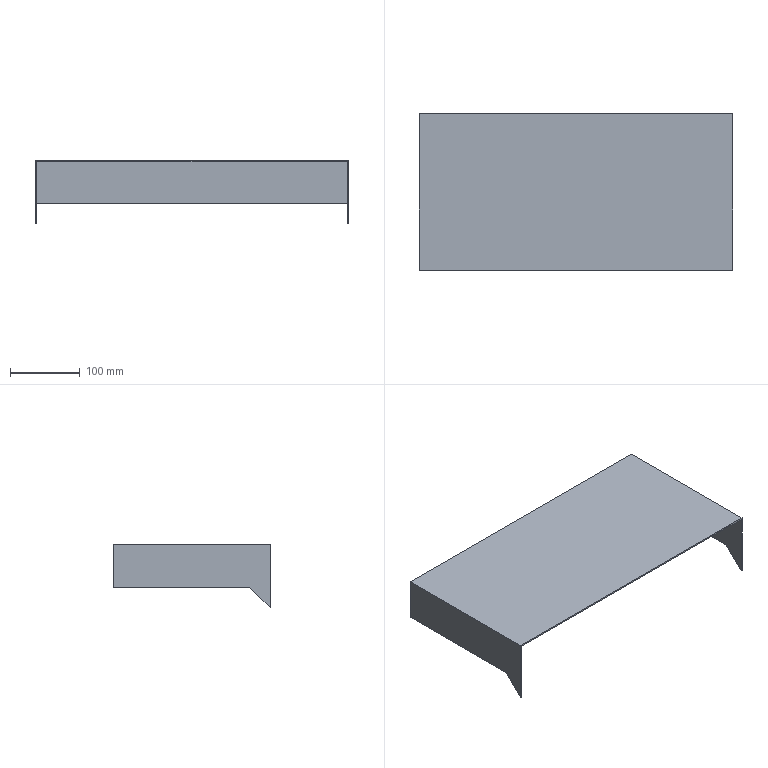Part | Creo | features PROTRUSION 5, CURVE 4, DATUM PLANE 3, COORDINATE SYSTEM 1, MIRROR 1 | 1 solid | 12 faces | box 450 x 225 x 92 mm | volume 311820 mm3 | plane 12
STEP:
#1=CARTESIAN_POINT('',(0.,0.,0.));
#2=DIRECTION('',(0.,0.,1.));
#3=DIRECTION('',(1.,0.,0.));
#4=AXIS2_PLACEMENT_3D('',#1,#2,#3);
#5=CARTESIAN_POINT('',(-223.,95.5,0.));
#6=VERTEX_POINT('',#5);
#7=CARTESIAN_POINT('',(-223.,-127.5,0.));
#8=VERTEX_POINT('',#7);
#9=CARTESIAN_POINT('',(-223.,95.5,0.));
#10=DIRECTION('',(0.,-1.,0.));
#11=VECTOR('',#10,223.);
#12=LINE('',#9,#11);
#13=EDGE_CURVE('',#6,#8,#12,.T.);
#14=ORIENTED_EDGE('',*,*,#13,.T.);
#15=CARTESIAN_POINT('',(223.,-127.5,0.));
#16=VERTEX_POINT('',#15);
#17=CARTESIAN_POINT('',(-223.,-127.5,0.));
#18=DIRECTION('',(1.,0.,0.));
#19=VECTOR('',#18,446.);
#20=LINE('',#17,#19);
#21=EDGE_CURVE('',#8,#16,#20,.T.);
#22=ORIENTED_EDGE('',*,*,#21,.T.);
#23=CARTESIAN_POINT('',(223.,95.5,0.));
#24=VERTEX_POINT('',#23);
#25=CARTESIAN_POINT('',(223.,-127.5,0.));
#26=DIRECTION('',(0.,1.,0.));
#27=VECTOR('',#26,223.);
#28=LINE('',#25,#27);
#29=EDGE_CURVE('',#16,#24,#28,.T.);
#30=ORIENTED_EDGE('',*,*,#29,.T.);
#31=CARTESIAN_POINT('',(223.,95.5,0.));
#32=DIRECTION('',(-1.,0.,0.));
#33=VECTOR('',#32,446.);
#34=LINE('',#31,#33);
#35=EDGE_CURVE('',#24,#6,#34,.T.);
#36=ORIENTED_EDGE('',*,*,#35,.T.);
#37=EDGE_LOOP('',(#14,#22,#30,#36));
#38=FACE_OUTER_BOUND('',#37,.F.);
#39=CARTESIAN_POINT('',(0.,0.,0.));
#40=DIRECTION('',(0.,0.,1.));
#41=DIRECTION('',(1.,0.,0.));
#42=AXIS2_PLACEMENT_3D('',#39,#40,#41);
#43=PLANE('',#42);
#44=ADVANCED_FACE('',(#38),#43,.F.);
#45=ORIENTED_EDGE('',*,*,#13,.F.);
#46=CARTESIAN_POINT('',(-223.,95.5,-60.));
#47=VERTEX_POINT('',#46);
#48=CARTESIAN_POINT('',(-223.,95.5,0.));
#49=DIRECTION('',(0.,0.,-1.));
#50=VECTOR('',#49,60.);
#51=LINE('',#48,#50);
#52=EDGE_CURVE('',#6,#47,#51,.T.);
#53=ORIENTED_EDGE('',*,*,#52,.T.);
#54=CARTESIAN_POINT('',(-223.,-97.5,-60.));
#55=VERTEX_POINT('',#54);
#56=CARTESIAN_POINT('',(-223.,95.5,-60.));
#57=DIRECTION('',(0.,-1.,0.));
#58=VECTOR('',#57,193.);
#59=LINE('',#56,#58);
#60=EDGE_CURVE('',#47,#55,#59,.T.);
#61=ORIENTED_EDGE('',*,*,#60,.T.);
#62=CARTESIAN_POINT('',(-223.,-127.5,-90.));
#63=VERTEX_POINT('',#62);
#64=CARTESIAN_POINT('',(-223.,-97.5,-60.));
#65=DIRECTION('',(0.,-0.7071,-0.7071));
#66=VECTOR('',#65,42.426);
#67=LINE('',#64,#66);
#68=EDGE_CURVE('',#55,#63,#67,.T.);
#69=ORIENTED_EDGE('',*,*,#68,.T.);
#70=CARTESIAN_POINT('',(-223.,-127.5,-90.));
#71=DIRECTION('',(0.,0.,1.));
#72=VECTOR('',#71,90.);
#73=LINE('',#70,#72);
#74=EDGE_CURVE('',#63,#8,#73,.T.);
#75=ORIENTED_EDGE('',*,*,#74,.T.);
#76=EDGE_LOOP('',(#45,#53,#61,#69,#75));
#77=FACE_OUTER_BOUND('',#76,.F.);
#78=CARTESIAN_POINT('',(-223.,95.5,0.));
#79=DIRECTION('',(1.,0.,0.));
#80=DIRECTION('',(0.,-1.,0.));
#81=AXIS2_PLACEMENT_3D('',#78,#79,#80);
#82=PLANE('',#81);
#83=ADVANCED_FACE('',(#77),#82,.T.);
#84=ORIENTED_EDGE('',*,*,#35,.F.);
#85=CARTESIAN_POINT('',(223.,95.5,-60.));
#86=VERTEX_POINT('',#85);
#87=CARTESIAN_POINT('',(223.,95.5,0.));
#88=DIRECTION('',(0.,0.,-1.));
#89=VECTOR('',#88,60.);
#90=LINE('',#87,#89);
#91=EDGE_CURVE('',#24,#86,#90,.T.);
#92=ORIENTED_EDGE('',*,*,#91,.T.);
#93=CARTESIAN_POINT('',(223.,95.5,-60.));
#94=DIRECTION('',(-1.,0.,0.));
#95=VECTOR('',#94,446.);
#96=LINE('',#93,#95);
#97=EDGE_CURVE('',#86,#47,#96,.T.);
#98=ORIENTED_EDGE('',*,*,#97,.T.);
#99=ORIENTED_EDGE('',*,*,#52,.F.);
#100=EDGE_LOOP('',(#84,#92,#98,#99));
#101=FACE_OUTER_BOUND('',#100,.F.);
#102=CARTESIAN_POINT('',(223.,95.5,0.));
#103=DIRECTION('',(0.,-1.,0.));
#104=DIRECTION('',(-1.,0.,0.));
#105=AXIS2_PLACEMENT_3D('',#102,#103,#104);
#106=PLANE('',#105);
#107=ADVANCED_FACE('',(#101),#106,.T.);
#108=ORIENTED_EDGE('',*,*,#29,.F.);
#109=CARTESIAN_POINT('',(223.,-127.5,-90.));
#110=VERTEX_POINT('',#109);
#111=CARTESIAN_POINT('',(223.,-127.5,-90.));
#112=DIRECTION('',(0.,0.,1.));
#113=VECTOR('',#112,90.);
#114=LINE('',#111,#113);
#115=EDGE_CURVE('',#110,#16,#114,.T.);
#116=ORIENTED_EDGE('',*,*,#115,.F.);
#117=CARTESIAN_POINT('',(223.,-97.5,-60.));
#118=VERTEX_POINT('',#117);
#119=CARTESIAN_POINT('',(223.,-97.5,-60.));
#120=DIRECTION('',(0.,-0.7071,-0.7071));
#121=VECTOR('',#120,42.426);
#122=LINE('',#119,#121);
#123=EDGE_CURVE('',#118,#110,#122,.T.);
#124=ORIENTED_EDGE('',*,*,#123,.F.);
#125=CARTESIAN_POINT('',(223.,-97.5,-60.));
#126=DIRECTION('',(0.,1.,0.));
#127=VECTOR('',#126,193.);
#128=LINE('',#125,#127);
#129=EDGE_CURVE('',#118,#86,#128,.T.);
#130=ORIENTED_EDGE('',*,*,#129,.T.);
#131=ORIENTED_EDGE('',*,*,#91,.F.);
#132=EDGE_LOOP('',(#108,#116,#124,#130,#131));
#133=FACE_OUTER_BOUND('',#132,.F.);
#134=CARTESIAN_POINT('',(223.,-97.5,0.));
#135=DIRECTION('',(-1.,0.,0.));
#136=DIRECTION('',(0.,1.,0.));
#137=AXIS2_PLACEMENT_3D('',#134,#135,#136);
#138=PLANE('',#137);
#139=ADVANCED_FACE('',(#133),#138,.T.);
#140=CARTESIAN_POINT('',(-225.,-127.5,2.));
#141=VERTEX_POINT('',#140);
#142=CARTESIAN_POINT('',(225.,-127.5,2.));
#143=VERTEX_POINT('',#142);
#144=CARTESIAN_POINT('',(-225.,-127.5,2.));
#145=DIRECTION('',(1.,0.,0.));
#146=VECTOR('',#145,450.);
#147=LINE('',#144,#146);
#148=EDGE_CURVE('',#141,#143,#147,.T.);
#149=ORIENTED_EDGE('',*,*,#148,.T.);
#150=CARTESIAN_POINT('',(225.,-127.5,-90.));
#151=VERTEX_POINT('',#150);
#152=CARTESIAN_POINT('',(225.,-127.5,-90.));
#153=DIRECTION('',(0.,0.,1.));
#154=VECTOR('',#153,92.);
#155=LINE('',#152,#154);
#156=EDGE_CURVE('',#151,#143,#155,.T.);
#157=ORIENTED_EDGE('',*,*,#156,.F.);
#158=CARTESIAN_POINT('',(225.,-127.5,-90.));
#159=DIRECTION('',(-1.,0.,0.));
#160=VECTOR('',#159,2.);
#161=LINE('',#158,#160);
#162=EDGE_CURVE('',#151,#110,#161,.T.);
#163=ORIENTED_EDGE('',*,*,#162,.T.);
#164=ORIENTED_EDGE('',*,*,#115,.T.);
#165=ORIENTED_EDGE('',*,*,#21,.F.);
#166=ORIENTED_EDGE('',*,*,#74,.F.);
#167=CARTESIAN_POINT('',(-225.,-127.5,-90.));
#168=VERTEX_POINT('',#167);
#169=CARTESIAN_POINT('',(-225.,-127.5,-90.));
#170=DIRECTION('',(1.,0.,0.));
#171=VECTOR('',#170,2.);
#172=LINE('',#169,#171);
#173=EDGE_CURVE('',#168,#63,#172,.T.);
#174=ORIENTED_EDGE('',*,*,#173,.F.);
#175=CARTESIAN_POINT('',(-225.,-127.5,-90.));
#176=DIRECTION('',(0.,0.,1.));
#177=VECTOR('',#176,92.);
#178=LINE('',#175,#177);
#179=EDGE_CURVE('',#168,#141,#178,.T.);
#180=ORIENTED_EDGE('',*,*,#179,.T.);
#181=EDGE_LOOP('',(#149,#157,#163,#164,#165,#166,#174,#180));
#182=FACE_OUTER_BOUND('',#181,.F.);
#183=CARTESIAN_POINT('',(-225.,-127.5,-90.));
#184=DIRECTION('',(0.,-1.,0.));
#185=DIRECTION('',(0.,0.,1.));
#186=AXIS2_PLACEMENT_3D('',#183,#184,#185);
#187=PLANE('',#186);
#188=ADVANCED_FACE('',(#182),#187,.T.);
#189=ORIENTED_EDGE('',*,*,#148,.F.);
#190=CARTESIAN_POINT('',(-225.,97.5,2.));
#191=VERTEX_POINT('',#190);
#192=CARTESIAN_POINT('',(-225.,-127.5,2.));
#193=DIRECTION('',(0.,1.,0.));
#194=VECTOR('',#193,225.);
#195=LINE('',#192,#194);
#196=EDGE_CURVE('',#141,#191,#195,.T.);
#197=ORIENTED_EDGE('',*,*,#196,.T.);
#198=CARTESIAN_POINT('',(225.,97.5,2.));
#199=VERTEX_POINT('',#198);
#200=CARTESIAN_POINT('',(225.,97.5,2.));
#201=DIRECTION('',(-1.,0.,0.));
#202=VECTOR('',#201,450.);
#203=LINE('',#200,#202);
#204=EDGE_CURVE('',#199,#191,#203,.T.);
#205=ORIENTED_EDGE('',*,*,#204,.F.);
#206=CARTESIAN_POINT('',(225.,97.5,2.));
#207=DIRECTION('',(0.,-1.,0.));
#208=VECTOR('',#207,225.);
#209=LINE('',#206,#208);
#210=EDGE_CURVE('',#199,#143,#209,.T.);
#211=ORIENTED_EDGE('',*,*,#210,.T.);
#212=EDGE_LOOP('',(#189,#197,#205,#211));
#213=FACE_OUTER_BOUND('',#212,.F.);
#214=CARTESIAN_POINT('',(0.,0.,2.));
#215=DIRECTION('',(0.,0.,1.));
#216=DIRECTION('',(1.,0.,0.));
#217=AXIS2_PLACEMENT_3D('',#214,#215,#216);
#218=PLANE('',#217);
#219=ADVANCED_FACE('',(#213),#218,.T.);
#220=ORIENTED_EDGE('',*,*,#196,.F.);
#221=ORIENTED_EDGE('',*,*,#179,.F.);
#222=CARTESIAN_POINT('',(-225.,-97.5,-60.));
#223=VERTEX_POINT('',#222);
#224=CARTESIAN_POINT('',(-225.,-97.5,-60.));
#225=DIRECTION('',(0.,-0.7071,-0.7071));
#226=VECTOR('',#225,42.426);
#227=LINE('',#224,#226);
#228=EDGE_CURVE('',#223,#168,#227,.T.);
#229=ORIENTED_EDGE('',*,*,#228,.F.);
#230=CARTESIAN_POINT('',(-225.,97.5,-60.));
#231=VERTEX_POINT('',#230);
#232=CARTESIAN_POINT('',(-225.,-97.5,-60.));
#233=DIRECTION('',(0.,1.,0.));
#234=VECTOR('',#233,195.);
#235=LINE('',#232,#234);
#236=EDGE_CURVE('',#223,#231,#235,.T.);
#237=ORIENTED_EDGE('',*,*,#236,.T.);
#238=CARTESIAN_POINT('',(-225.,97.5,2.));
#239=DIRECTION('',(0.,0.,-1.));
#240=VECTOR('',#239,62.);
#241=LINE('',#238,#240);
#242=EDGE_CURVE('',#191,#231,#241,.T.);
#243=ORIENTED_EDGE('',*,*,#242,.F.);
#244=EDGE_LOOP('',(#220,#221,#229,#237,#243));
#245=FACE_OUTER_BOUND('',#244,.F.);
#246=CARTESIAN_POINT('',(-225.,97.5,0.));
#247=DIRECTION('',(-1.,0.,0.));
#248=DIRECTION('',(0.,-1.,0.));
#249=AXIS2_PLACEMENT_3D('',#246,#247,#248);
#250=PLANE('',#249);
#251=ADVANCED_FACE('',(#245),#250,.T.);
#252=CARTESIAN_POINT('',(-225.,-97.5,-60.));
#253=DIRECTION('',(1.,0.,0.));
#254=VECTOR('',#253,2.);
#255=LINE('',#252,#254);
#256=EDGE_CURVE('',#223,#55,#255,.T.);
#257=ORIENTED_EDGE('',*,*,#256,.F.);
#258=ORIENTED_EDGE('',*,*,#228,.T.);
#259=ORIENTED_EDGE('',*,*,#173,.T.);
#260=ORIENTED_EDGE('',*,*,#68,.F.);
#261=EDGE_LOOP('',(#257,#258,#259,#260));
#262=FACE_OUTER_BOUND('',#261,.F.);
#263=CARTESIAN_POINT('',(-225.,-97.5,-60.));
#264=DIRECTION('',(0.,0.7071,-0.7071));
#265=DIRECTION('',(0.,-0.7071,-0.7071));
#266=AXIS2_PLACEMENT_3D('',#263,#264,#265);
#267=PLANE('',#266);
#268=ADVANCED_FACE('',(#262),#267,.T.);
#269=CARTESIAN_POINT('',(225.,-97.5,-60.));
#270=VERTEX_POINT('',#269);
#271=CARTESIAN_POINT('',(225.,-97.5,-60.));
#272=DIRECTION('',(-1.,0.,0.));
#273=VECTOR('',#272,2.);
#274=LINE('',#271,#273);
#275=EDGE_CURVE('',#270,#118,#274,.T.);
#276=ORIENTED_EDGE('',*,*,#275,.F.);
#277=CARTESIAN_POINT('',(225.,97.5,-60.));
#278=VERTEX_POINT('',#277);
#279=CARTESIAN_POINT('',(225.,97.5,-60.));
#280=DIRECTION('',(0.,-1.,0.));
#281=VECTOR('',#280,195.);
#282=LINE('',#279,#281);
#283=EDGE_CURVE('',#278,#270,#282,.T.);
#284=ORIENTED_EDGE('',*,*,#283,.F.);
#285=CARTESIAN_POINT('',(-225.,97.5,-60.));
#286=DIRECTION('',(1.,0.,0.));
#287=VECTOR('',#286,450.);
#288=LINE('',#285,#287);
#289=EDGE_CURVE('',#231,#278,#288,.T.);
#290=ORIENTED_EDGE('',*,*,#289,.F.);
#291=ORIENTED_EDGE('',*,*,#236,.F.);
#292=ORIENTED_EDGE('',*,*,#256,.T.);
#293=ORIENTED_EDGE('',*,*,#60,.F.);
#294=ORIENTED_EDGE('',*,*,#97,.F.);
#295=ORIENTED_EDGE('',*,*,#129,.F.);
#296=EDGE_LOOP('',(#276,#284,#290,#291,#292,#293,#294,#295));
#297=FACE_OUTER_BOUND('',#296,.F.);
#298=CARTESIAN_POINT('',(0.,0.,-60.));
#299=DIRECTION('',(0.,0.,-1.));
#300=DIRECTION('',(-1.,0.,0.));
#301=AXIS2_PLACEMENT_3D('',#298,#299,#300);
#302=PLANE('',#301);
#303=ADVANCED_FACE('',(#297),#302,.T.);
#304=CARTESIAN_POINT('',(225.,-97.5,-60.));
#305=DIRECTION('',(0.,-0.7071,-0.7071));
#306=VECTOR('',#305,42.426);
#307=LINE('',#304,#306);
#308=EDGE_CURVE('',#270,#151,#307,.T.);
#309=ORIENTED_EDGE('',*,*,#308,.F.);
#310=ORIENTED_EDGE('',*,*,#275,.T.);
#311=ORIENTED_EDGE('',*,*,#123,.T.);
#312=ORIENTED_EDGE('',*,*,#162,.F.);
#313=EDGE_LOOP('',(#309,#310,#311,#312));
#314=FACE_OUTER_BOUND('',#313,.F.);
#315=CARTESIAN_POINT('',(225.,-97.5,-60.));
#316=DIRECTION('',(0.,-0.7071,0.7071));
#317=DIRECTION('',(0.,-0.7071,-0.7071));
#318=AXIS2_PLACEMENT_3D('',#315,#316,#317);
#319=PLANE('',#318);
#320=ADVANCED_FACE('',(#314),#319,.F.);
#321=ORIENTED_EDGE('',*,*,#283,.T.);
#322=ORIENTED_EDGE('',*,*,#308,.T.);
#323=ORIENTED_EDGE('',*,*,#156,.T.);
#324=ORIENTED_EDGE('',*,*,#210,.F.);
#325=CARTESIAN_POINT('',(225.,97.5,2.));
#326=DIRECTION('',(0.,0.,-1.));
#327=VECTOR('',#326,62.);
#328=LINE('',#325,#327);
#329=EDGE_CURVE('',#199,#278,#328,.T.);
#330=ORIENTED_EDGE('',*,*,#329,.T.);
#331=EDGE_LOOP('',(#321,#322,#323,#324,#330));
#332=FACE_OUTER_BOUND('',#331,.F.);
#333=CARTESIAN_POINT('',(225.,-97.5,0.));
#334=DIRECTION('',(1.,0.,0.));
#335=DIRECTION('',(0.,1.,0.));
#336=AXIS2_PLACEMENT_3D('',#333,#334,#335);
#337=PLANE('',#336);
#338=ADVANCED_FACE('',(#332),#337,.T.);
#339=ORIENTED_EDGE('',*,*,#242,.T.);
#340=ORIENTED_EDGE('',*,*,#289,.T.);
#341=ORIENTED_EDGE('',*,*,#329,.F.);
#342=ORIENTED_EDGE('',*,*,#204,.T.);
#343=EDGE_LOOP('',(#339,#340,#341,#342));
#344=FACE_OUTER_BOUND('',#343,.F.);
#345=CARTESIAN_POINT('',(225.,97.5,0.));
#346=DIRECTION('',(0.,1.,0.));
#347=DIRECTION('',(-1.,0.,0.));
#348=AXIS2_PLACEMENT_3D('',#345,#346,#347);
#349=PLANE('',#348);
#350=ADVANCED_FACE('',(#344),#349,.T.);
#351=CLOSED_SHELL('',(#44,#83,#107,#139,#188,#219,#251,#268,#303,#320,#338,#350));
#352=MANIFOLD_SOLID_BREP('',#351);
#353=(LENGTH_UNIT()NAMED_UNIT(*)SI_UNIT(.MILLI.,.METRE.));
#354=UNCERTAINTY_MEASURE_WITH_UNIT(LENGTH_MEASURE(0.05114),#353,'','');
#355=(NAMED_UNIT(*)PLANE_ANGLE_UNIT()SI_UNIT($,.RADIAN.));
#356=PLANE_ANGLE_MEASURE_WITH_UNIT(PLANE_ANGLE_MEASURE(0.01745),#355);
#357=(CONVERSION_BASED_UNIT('DEGREE',#356)NAMED_UNIT(*)PLANE_ANGLE_UNIT());
#358=(NAMED_UNIT(*)SI_UNIT($,.STERADIAN.)SOLID_ANGLE_UNIT());
#359=(GEOMETRIC_REPRESENTATION_CONTEXT(3)GLOBAL_UNCERTAINTY_ASSIGNED_CONTEXT((#354))GLOBAL_UNIT_ASSIGNED_CONTEXT((#353,#357,#358))REPRESENTATION_CONTEXT('',''));
#360=ADVANCED_BREP_SHAPE_REPRESENTATION('',(#4,#352),#359);